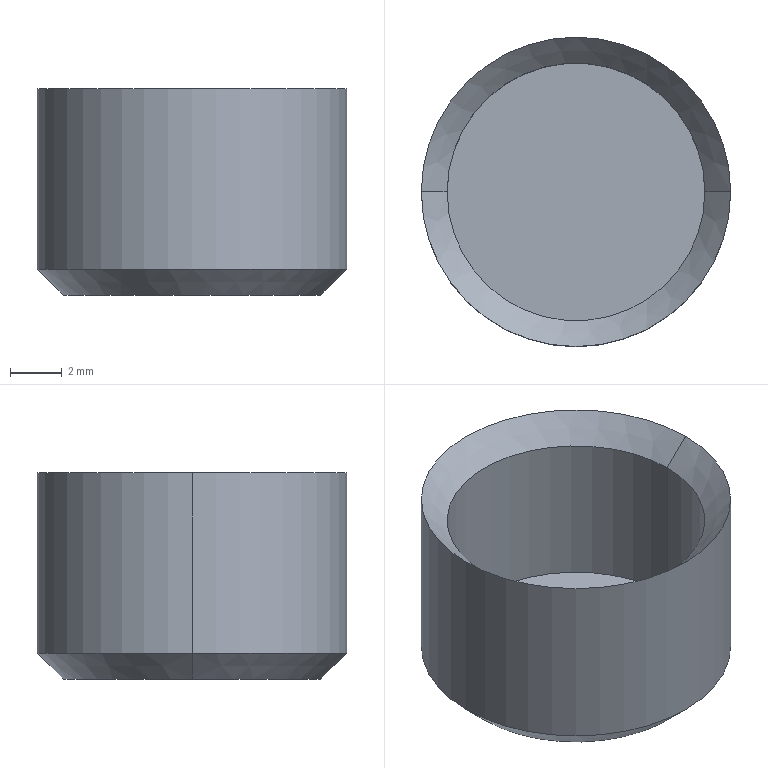Part | SolidWorks | features Chamfer 1, Extrusion 1, ICE 1 | 1 solid | 10 faces | box 12 x 12 x 8 mm | volume 320.442 mm3 | cone 4 | cylinder 4 | plane 2 | commonest cylinder face diameters 10 x2 12 x2
STEP:
#1=CARTESIAN_POINT('',(-5.,0.,0.));
#2=VERTEX_POINT('',#1);
#3=CARTESIAN_POINT('',(5.,0.,0.));
#4=VERTEX_POINT('',#3);
#5=CARTESIAN_POINT('',(0.,0.,0.));
#6=DIRECTION('',(0.,0.,-1.));
#7=DIRECTION('',(1.,0.,0.));
#8=AXIS2_PLACEMENT_3D('',#5,#6,#7);
#9=CIRCLE('',#8,5.);
#10=EDGE_CURVE('',#2,#4,#9,.T.);
#11=ORIENTED_EDGE('',*,*,#10,.F.);
#12=CARTESIAN_POINT('',(-6.,0.,1.));
#13=VERTEX_POINT('',#12);
#14=CARTESIAN_POINT('',(-6.,0.,1.));
#15=DIRECTION('',(-0.7071,0.,0.7071));
#16=VECTOR('',#15,1000.);
#17=LINE('',#14,#16);
#18=EDGE_CURVE('',#2,#13,#17,.T.);
#19=ORIENTED_EDGE('',*,*,#18,.T.);
#20=CARTESIAN_POINT('',(6.,0.,1.));
#21=VERTEX_POINT('',#20);
#22=CARTESIAN_POINT('',(0.,0.,1.));
#23=DIRECTION('',(0.,0.,1.));
#24=DIRECTION('',(1.,0.,0.));
#25=AXIS2_PLACEMENT_3D('',#22,#23,#24);
#26=CIRCLE('',#25,6.);
#27=EDGE_CURVE('',#21,#13,#26,.T.);
#28=ORIENTED_EDGE('',*,*,#27,.F.);
#29=CARTESIAN_POINT('',(6.,0.,1.));
#30=DIRECTION('',(0.7071,0.,0.7071));
#31=VECTOR('',#30,1000.);
#32=LINE('',#29,#31);
#33=EDGE_CURVE('',#4,#21,#32,.T.);
#34=ORIENTED_EDGE('',*,*,#33,.F.);
#35=EDGE_LOOP('',(#11,#19,#28,#34));
#36=FACE_OUTER_BOUND('',#35,.T.);
#37=CARTESIAN_POINT('',(0.,0.,1.));
#38=DIRECTION('',(0.,0.,1.));
#39=DIRECTION('',(1.,0.,0.));
#40=AXIS2_PLACEMENT_3D('',#37,#38,#39);
#41=CONICAL_SURFACE('',#40,6.,0.7854);
#42=ADVANCED_FACE('',(#36),#41,.T.);
#43=CARTESIAN_POINT('',(-5.,0.,7.));
#44=VERTEX_POINT('',#43);
#45=CARTESIAN_POINT('',(5.,0.,7.));
#46=VERTEX_POINT('',#45);
#47=CARTESIAN_POINT('',(0.,0.,7.));
#48=DIRECTION('',(0.,0.,1.));
#49=DIRECTION('',(1.,0.,0.));
#50=AXIS2_PLACEMENT_3D('',#47,#48,#49);
#51=CIRCLE('',#50,5.);
#52=EDGE_CURVE('',#44,#46,#51,.T.);
#53=ORIENTED_EDGE('',*,*,#52,.F.);
#54=CARTESIAN_POINT('',(-6.,0.,8.));
#55=VERTEX_POINT('',#54);
#56=CARTESIAN_POINT('',(-5.,0.,7.));
#57=DIRECTION('',(-0.7071,0.,0.7071));
#58=VECTOR('',#57,1000.);
#59=LINE('',#56,#58);
#60=EDGE_CURVE('',#44,#55,#59,.T.);
#61=ORIENTED_EDGE('',*,*,#60,.T.);
#62=CARTESIAN_POINT('',(6.,0.,8.));
#63=VERTEX_POINT('',#62);
#64=CARTESIAN_POINT('',(0.,0.,8.));
#65=DIRECTION('',(0.,0.,1.));
#66=DIRECTION('',(1.,0.,0.));
#67=AXIS2_PLACEMENT_3D('',#64,#65,#66);
#68=CIRCLE('',#67,6.);
#69=EDGE_CURVE('',#55,#63,#68,.T.);
#70=ORIENTED_EDGE('',*,*,#69,.T.);
#71=CARTESIAN_POINT('',(5.,0.,7.));
#72=DIRECTION('',(0.7071,0.,0.7071));
#73=VECTOR('',#72,1000.);
#74=LINE('',#71,#73);
#75=EDGE_CURVE('',#46,#63,#74,.T.);
#76=ORIENTED_EDGE('',*,*,#75,.F.);
#77=EDGE_LOOP('',(#53,#61,#70,#76));
#78=FACE_OUTER_BOUND('',#77,.T.);
#79=CARTESIAN_POINT('',(0.,0.,7.));
#80=DIRECTION('',(0.,0.,1.));
#81=DIRECTION('',(1.,0.,0.));
#82=AXIS2_PLACEMENT_3D('',#79,#80,#81);
#83=CONICAL_SURFACE('',#82,5.,0.7854);
#84=ADVANCED_FACE('',(#78),#83,.F.);
#85=CARTESIAN_POINT('',(-5.,0.,1.));
#86=VERTEX_POINT('',#85);
#87=CARTESIAN_POINT('',(5.,0.,1.));
#88=VERTEX_POINT('',#87);
#89=CARTESIAN_POINT('',(0.,0.,1.));
#90=DIRECTION('',(0.,0.,1.));
#91=DIRECTION('',(1.,0.,0.));
#92=AXIS2_PLACEMENT_3D('',#89,#90,#91);
#93=CIRCLE('',#92,5.);
#94=EDGE_CURVE('',#86,#88,#93,.T.);
#95=ORIENTED_EDGE('',*,*,#94,.F.);
#96=CARTESIAN_POINT('',(-5.,0.,1.));
#97=DIRECTION('',(0.,0.,1.));
#98=VECTOR('',#97,1000.);
#99=LINE('',#96,#98);
#100=EDGE_CURVE('',#86,#44,#99,.T.);
#101=ORIENTED_EDGE('',*,*,#100,.T.);
#102=ORIENTED_EDGE('',*,*,#52,.T.);
#103=CARTESIAN_POINT('',(5.,0.,1.));
#104=DIRECTION('',(0.,0.,1.));
#105=VECTOR('',#104,1000.);
#106=LINE('',#103,#105);
#107=EDGE_CURVE('',#88,#46,#106,.T.);
#108=ORIENTED_EDGE('',*,*,#107,.F.);
#109=EDGE_LOOP('',(#95,#101,#102,#108));
#110=FACE_OUTER_BOUND('',#109,.T.);
#111=CARTESIAN_POINT('',(0.,0.,1.));
#112=DIRECTION('',(0.,0.,1.));
#113=DIRECTION('',(1.,0.,0.));
#114=AXIS2_PLACEMENT_3D('',#111,#112,#113);
#115=CYLINDRICAL_SURFACE('',#114,5.);
#116=ADVANCED_FACE('',(#110),#115,.F.);
#117=CARTESIAN_POINT('',(0.,0.,8.));
#118=DIRECTION('',(0.,0.,1.));
#119=DIRECTION('',(1.,0.,0.));
#120=AXIS2_PLACEMENT_3D('',#117,#118,#119);
#121=CIRCLE('',#120,6.);
#122=EDGE_CURVE('',#63,#55,#121,.T.);
#123=ORIENTED_EDGE('',*,*,#122,.F.);
#124=CARTESIAN_POINT('',(6.,0.,8.));
#125=DIRECTION('',(0.,0.,-1.));
#126=VECTOR('',#125,1000.);
#127=LINE('',#124,#126);
#128=EDGE_CURVE('',#63,#21,#127,.T.);
#129=ORIENTED_EDGE('',*,*,#128,.T.);
#130=ORIENTED_EDGE('',*,*,#27,.T.);
#131=CARTESIAN_POINT('',(-6.,0.,8.));
#132=DIRECTION('',(0.,0.,-1.));
#133=VECTOR('',#132,1000.);
#134=LINE('',#131,#133);
#135=EDGE_CURVE('',#55,#13,#134,.T.);
#136=ORIENTED_EDGE('',*,*,#135,.F.);
#137=EDGE_LOOP('',(#123,#129,#130,#136));
#138=FACE_OUTER_BOUND('',#137,.T.);
#139=CARTESIAN_POINT('',(0.,0.,8.));
#140=DIRECTION('',(0.,0.,-1.));
#141=DIRECTION('',(-1.,0.,0.));
#142=AXIS2_PLACEMENT_3D('',#139,#140,#141);
#143=CYLINDRICAL_SURFACE('',#142,6.);
#144=ADVANCED_FACE('',(#138),#143,.T.);
#145=ORIENTED_EDGE('',*,*,#128,.F.);
#146=ORIENTED_EDGE('',*,*,#69,.F.);
#147=ORIENTED_EDGE('',*,*,#135,.T.);
#148=CARTESIAN_POINT('',(0.,0.,1.));
#149=DIRECTION('',(0.,0.,1.));
#150=DIRECTION('',(1.,0.,0.));
#151=AXIS2_PLACEMENT_3D('',#148,#149,#150);
#152=CIRCLE('',#151,6.);
#153=EDGE_CURVE('',#13,#21,#152,.T.);
#154=ORIENTED_EDGE('',*,*,#153,.T.);
#155=EDGE_LOOP('',(#145,#146,#147,#154));
#156=FACE_OUTER_BOUND('',#155,.T.);
#157=CARTESIAN_POINT('',(0.,0.,8.));
#158=DIRECTION('',(0.,0.,-1.));
#159=DIRECTION('',(-1.,0.,0.));
#160=AXIS2_PLACEMENT_3D('',#157,#158,#159);
#161=CYLINDRICAL_SURFACE('',#160,6.);
#162=ADVANCED_FACE('',(#156),#161,.T.);
#163=CARTESIAN_POINT('',(0.,0.,0.));
#164=DIRECTION('',(0.,0.,-1.));
#165=DIRECTION('',(1.,0.,0.));
#166=AXIS2_PLACEMENT_3D('',#163,#164,#165);
#167=CIRCLE('',#166,5.);
#168=EDGE_CURVE('',#4,#2,#167,.T.);
#169=ORIENTED_EDGE('',*,*,#168,.T.);
#170=ORIENTED_EDGE('',*,*,#10,.T.);
#171=EDGE_LOOP('',(#169,#170));
#172=FACE_OUTER_BOUND('',#171,.T.);
#173=CARTESIAN_POINT('',(0.,0.,0.));
#174=DIRECTION('',(0.,0.,1.));
#175=DIRECTION('',(1.,0.,0.));
#176=AXIS2_PLACEMENT_3D('',#173,#174,#175);
#177=PLANE('',#176);
#178=ADVANCED_FACE('',(#172),#177,.F.);
#179=ORIENTED_EDGE('',*,*,#100,.F.);
#180=CARTESIAN_POINT('',(0.,0.,1.));
#181=DIRECTION('',(0.,0.,1.));
#182=DIRECTION('',(1.,0.,0.));
#183=AXIS2_PLACEMENT_3D('',#180,#181,#182);
#184=CIRCLE('',#183,5.);
#185=EDGE_CURVE('',#88,#86,#184,.T.);
#186=ORIENTED_EDGE('',*,*,#185,.F.);
#187=ORIENTED_EDGE('',*,*,#107,.T.);
#188=CARTESIAN_POINT('',(0.,0.,7.));
#189=DIRECTION('',(0.,0.,1.));
#190=DIRECTION('',(1.,0.,0.));
#191=AXIS2_PLACEMENT_3D('',#188,#189,#190);
#192=CIRCLE('',#191,5.);
#193=EDGE_CURVE('',#46,#44,#192,.T.);
#194=ORIENTED_EDGE('',*,*,#193,.T.);
#195=EDGE_LOOP('',(#179,#186,#187,#194));
#196=FACE_OUTER_BOUND('',#195,.T.);
#197=CARTESIAN_POINT('',(0.,0.,1.));
#198=DIRECTION('',(0.,0.,1.));
#199=DIRECTION('',(1.,0.,0.));
#200=AXIS2_PLACEMENT_3D('',#197,#198,#199);
#201=CYLINDRICAL_SURFACE('',#200,5.);
#202=ADVANCED_FACE('',(#196),#201,.F.);
#203=ORIENTED_EDGE('',*,*,#185,.T.);
#204=ORIENTED_EDGE('',*,*,#94,.T.);
#205=EDGE_LOOP('',(#203,#204));
#206=FACE_OUTER_BOUND('',#205,.T.);
#207=CARTESIAN_POINT('',(0.,0.,1.));
#208=DIRECTION('',(0.,0.,1.));
#209=DIRECTION('',(1.,0.,0.));
#210=AXIS2_PLACEMENT_3D('',#207,#208,#209);
#211=PLANE('',#210);
#212=ADVANCED_FACE('',(#206),#211,.T.);
#213=ORIENTED_EDGE('',*,*,#60,.F.);
#214=ORIENTED_EDGE('',*,*,#193,.F.);
#215=ORIENTED_EDGE('',*,*,#75,.T.);
#216=ORIENTED_EDGE('',*,*,#122,.T.);
#217=EDGE_LOOP('',(#213,#214,#215,#216));
#218=FACE_OUTER_BOUND('',#217,.T.);
#219=CARTESIAN_POINT('',(0.,0.,7.));
#220=DIRECTION('',(0.,0.,1.));
#221=DIRECTION('',(1.,0.,0.));
#222=AXIS2_PLACEMENT_3D('',#219,#220,#221);
#223=CONICAL_SURFACE('',#222,5.,0.7854);
#224=ADVANCED_FACE('',(#218),#223,.F.);
#225=ORIENTED_EDGE('',*,*,#18,.F.);
#226=ORIENTED_EDGE('',*,*,#168,.F.);
#227=ORIENTED_EDGE('',*,*,#33,.T.);
#228=ORIENTED_EDGE('',*,*,#153,.F.);
#229=EDGE_LOOP('',(#225,#226,#227,#228));
#230=FACE_OUTER_BOUND('',#229,.T.);
#231=CARTESIAN_POINT('',(0.,0.,1.));
#232=DIRECTION('',(0.,0.,1.));
#233=DIRECTION('',(1.,0.,0.));
#234=AXIS2_PLACEMENT_3D('',#231,#232,#233);
#235=CONICAL_SURFACE('',#234,6.,0.7854);
#236=ADVANCED_FACE('',(#230),#235,.T.);
#237=CLOSED_SHELL('',(#42,#84,#116,#144,#162,#178,#202,#212,#224,#236));
#238=MANIFOLD_SOLID_BREP('',#237);
#239=CARTESIAN_POINT('',(0.,0.,0.));
#240=DIRECTION('',(0.,0.,1.));
#241=DIRECTION('',(1.,0.,0.));
#242=AXIS2_PLACEMENT_3D('',#239,#240,#241);
#243=(LENGTH_UNIT()NAMED_UNIT(*)SI_UNIT(.MILLI.,.METRE.));
#244=UNCERTAINTY_MEASURE_WITH_UNIT(LENGTH_MEASURE(0.00001),#243,'','');
#245=(NAMED_UNIT(*)PLANE_ANGLE_UNIT()SI_UNIT($,.RADIAN.));
#246=(NAMED_UNIT(*)SI_UNIT($,.STERADIAN.)SOLID_ANGLE_UNIT());
#247=(GEOMETRIC_REPRESENTATION_CONTEXT(3)GLOBAL_UNCERTAINTY_ASSIGNED_CONTEXT((#244))GLOBAL_UNIT_ASSIGNED_CONTEXT((#243,#245,#246))REPRESENTATION_CONTEXT('',''));
#248=ADVANCED_BREP_SHAPE_REPRESENTATION('',(#238,#242),#247);